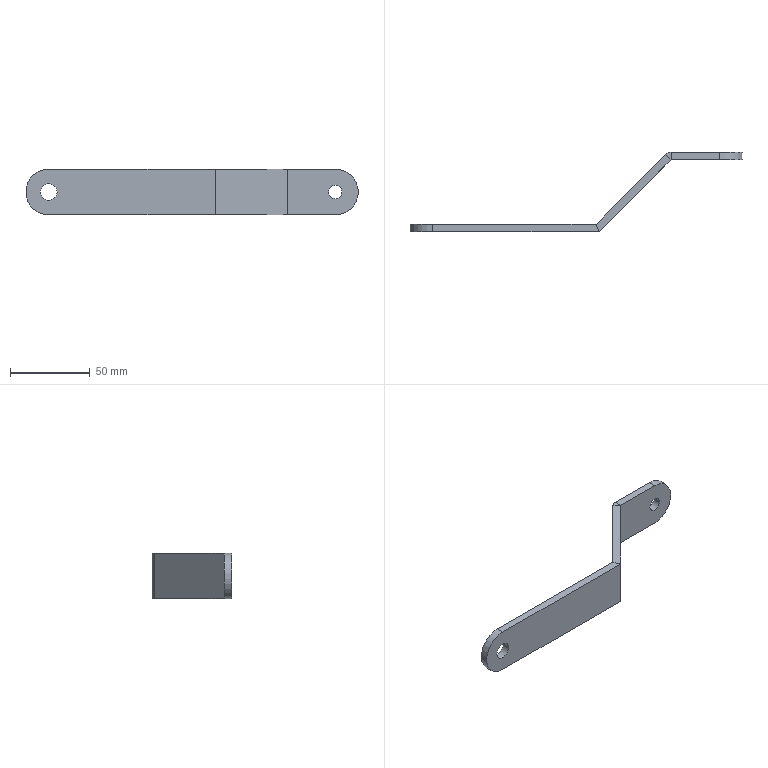Part | NX | features BREP 1 | 1 solid | 21 faces | box 207.715 x 49.664 x 28.575 mm | volume 29293 mm3 | plane 14 | cylinder 7 | commonest cylinder face diameters 8.204 x2 10.414 x2 28.575 x2 9.525 x1
STEP:
#1=CARTESIAN_POINT('',(118.364,0.,14.287));
#2=VERTEX_POINT('',#1);
#3=CARTESIAN_POINT('',(118.364,0.,-14.287));
#4=VERTEX_POINT('',#3);
#5=CARTESIAN_POINT('',(118.364,0.,14.287));
#6=DIRECTION('',(0.,0.,-1.));
#7=VECTOR('',#6,1000.);
#8=LINE('',#5,#7);
#9=EDGE_CURVE('',#2,#4,#8,.T.);
#10=ORIENTED_EDGE('',*,*,#9,.T.);
#11=CARTESIAN_POINT('',(163.265,44.901,-14.287));
#12=VERTEX_POINT('',#11);
#13=CARTESIAN_POINT('',(118.364,0.,-14.287));
#14=DIRECTION('',(0.7071,0.7071,0.));
#15=VECTOR('',#14,1000.);
#16=LINE('',#13,#15);
#17=EDGE_CURVE('',#4,#12,#16,.T.);
#18=ORIENTED_EDGE('',*,*,#17,.T.);
#19=CARTESIAN_POINT('',(163.265,44.901,14.287));
#20=VERTEX_POINT('',#19);
#21=CARTESIAN_POINT('',(163.265,44.901,14.287));
#22=DIRECTION('',(0.,0.,-1.));
#23=VECTOR('',#22,1000.);
#24=LINE('',#21,#23);
#25=EDGE_CURVE('',#20,#12,#24,.T.);
#26=ORIENTED_EDGE('',*,*,#25,.F.);
#27=CARTESIAN_POINT('',(118.364,0.,14.287));
#28=DIRECTION('',(0.7071,0.7071,0.));
#29=VECTOR('',#28,1000.);
#30=LINE('',#27,#29);
#31=EDGE_CURVE('',#2,#20,#30,.T.);
#32=ORIENTED_EDGE('',*,*,#31,.F.);
#33=EDGE_LOOP('',(#10,#18,#26,#32));
#34=FACE_BOUND('',#33,.T.);
#35=CARTESIAN_POINT('',(118.364,0.,14.287));
#36=DIRECTION('',(0.7071,-0.7071,0.));
#37=DIRECTION('',(0.,0.,-1.));
#38=AXIS2_PLACEMENT_3D('',#35,#36,#37);
#39=PLANE('',#38);
#40=ADVANCED_FACE('',(#34),#39,.T.);
#41=CARTESIAN_POINT('',(159.898,48.269,14.287));
#42=VERTEX_POINT('',#41);
#43=CARTESIAN_POINT('',(163.265,44.901,14.287));
#44=DIRECTION('',(-0.7071,0.7071,0.));
#45=VECTOR('',#44,1000.);
#46=LINE('',#43,#45);
#47=EDGE_CURVE('',#20,#42,#46,.T.);
#48=ORIENTED_EDGE('',*,*,#47,.T.);
#49=CARTESIAN_POINT('',(116.391,4.763,14.287));
#50=VERTEX_POINT('',#49);
#51=CARTESIAN_POINT('',(116.391,4.763,14.287));
#52=DIRECTION('',(0.7071,0.7071,0.));
#53=VECTOR('',#52,1000.);
#54=LINE('',#51,#53);
#55=EDGE_CURVE('',#50,#42,#54,.T.);
#56=ORIENTED_EDGE('',*,*,#55,.F.);
#57=CARTESIAN_POINT('',(118.364,0.,14.287));
#58=DIRECTION('',(-0.3827,0.9239,0.));
#59=VECTOR('',#58,1000.);
#60=LINE('',#57,#59);
#61=EDGE_CURVE('',#2,#50,#60,.T.);
#62=ORIENTED_EDGE('',*,*,#61,.F.);
#63=ORIENTED_EDGE('',*,*,#31,.T.);
#64=EDGE_LOOP('',(#48,#56,#62,#63));
#65=FACE_BOUND('',#64,.T.);
#66=CARTESIAN_POINT('',(139.48,24.483,14.287));
#67=DIRECTION('',(0.,0.,-1.));
#68=DIRECTION('',(0.,-1.,0.));
#69=AXIS2_PLACEMENT_3D('',#66,#67,#68);
#70=PLANE('',#69);
#71=ADVANCED_FACE('',(#65),#70,.F.);
#72=CARTESIAN_POINT('',(14.287,0.,14.287));
#73=VERTEX_POINT('',#72);
#74=CARTESIAN_POINT('',(14.287,0.,14.287));
#75=DIRECTION('',(1.,0.,0.));
#76=VECTOR('',#75,1000.);
#77=LINE('',#74,#76);
#78=EDGE_CURVE('',#73,#2,#77,.T.);
#79=ORIENTED_EDGE('',*,*,#78,.T.);
#80=ORIENTED_EDGE('',*,*,#61,.T.);
#81=CARTESIAN_POINT('',(14.287,4.763,14.287));
#82=VERTEX_POINT('',#81);
#83=CARTESIAN_POINT('',(14.287,4.763,14.287));
#84=DIRECTION('',(1.,0.,0.));
#85=VECTOR('',#84,1000.);
#86=LINE('',#83,#85);
#87=EDGE_CURVE('',#82,#50,#86,.T.);
#88=ORIENTED_EDGE('',*,*,#87,.F.);
#89=CARTESIAN_POINT('',(14.287,0.,14.287));
#90=DIRECTION('',(0.,1.,0.));
#91=VECTOR('',#90,1000.);
#92=LINE('',#89,#91);
#93=EDGE_CURVE('',#73,#82,#92,.T.);
#94=ORIENTED_EDGE('',*,*,#93,.F.);
#95=EDGE_LOOP('',(#79,#80,#88,#94));
#96=FACE_BOUND('',#95,.T.);
#97=CARTESIAN_POINT('',(58.689,2.381,14.287));
#98=DIRECTION('',(0.,0.,-1.));
#99=DIRECTION('',(0.,-1.,0.));
#100=AXIS2_PLACEMENT_3D('',#97,#98,#99);
#101=PLANE('',#100);
#102=ADVANCED_FACE('',(#96),#101,.F.);
#103=CARTESIAN_POINT('',(14.287,4.763,-14.287));
#104=VERTEX_POINT('',#103);
#105=CARTESIAN_POINT('',(14.287,4.763,0.));
#106=DIRECTION('',(0.,1.,0.));
#107=DIRECTION('',(0.,0.,-1.));
#108=AXIS2_PLACEMENT_3D('',#105,#106,#107);
#109=CIRCLE('',#108,14.287);
#110=EDGE_CURVE('',#104,#82,#109,.T.);
#111=ORIENTED_EDGE('',*,*,#110,.F.);
#112=CARTESIAN_POINT('',(14.287,0.,-14.287));
#113=VERTEX_POINT('',#112);
#114=CARTESIAN_POINT('',(14.287,0.,-14.287));
#115=DIRECTION('',(0.,1.,0.));
#116=VECTOR('',#115,1000.);
#117=LINE('',#114,#116);
#118=EDGE_CURVE('',#113,#104,#117,.T.);
#119=ORIENTED_EDGE('',*,*,#118,.F.);
#120=CARTESIAN_POINT('',(14.287,0.,0.));
#121=DIRECTION('',(0.,-1.,0.));
#122=DIRECTION('',(0.,0.,1.));
#123=AXIS2_PLACEMENT_3D('',#120,#121,#122);
#124=CIRCLE('',#123,14.287);
#125=EDGE_CURVE('',#73,#113,#124,.T.);
#126=ORIENTED_EDGE('',*,*,#125,.F.);
#127=ORIENTED_EDGE('',*,*,#93,.T.);
#128=EDGE_LOOP('',(#111,#119,#126,#127));
#129=FACE_BOUND('',#128,.T.);
#130=CARTESIAN_POINT('',(14.287,-0.3376,0.));
#131=DIRECTION('',(0.,1.,0.));
#132=DIRECTION('',(0.,0.,1.));
#133=AXIS2_PLACEMENT_3D('',#130,#131,#132);
#134=CYLINDRICAL_SURFACE('',#133,14.287);
#135=ADVANCED_FACE('',(#129),#134,.T.);
#136=CARTESIAN_POINT('',(14.287,0.,-14.287));
#137=DIRECTION('',(1.,0.,0.));
#138=VECTOR('',#137,1000.);
#139=LINE('',#136,#138);
#140=EDGE_CURVE('',#113,#4,#139,.T.);
#141=ORIENTED_EDGE('',*,*,#140,.T.);
#142=ORIENTED_EDGE('',*,*,#9,.F.);
#143=ORIENTED_EDGE('',*,*,#78,.F.);
#144=ORIENTED_EDGE('',*,*,#125,.T.);
#145=EDGE_LOOP('',(#141,#142,#143,#144));
#146=FACE_BOUND('',#145,.T.);
#147=CARTESIAN_POINT('',(19.494,0.,0.));
#148=VERTEX_POINT('',#147);
#149=CARTESIAN_POINT('',(9.081,0.,0.));
#150=VERTEX_POINT('',#149);
#151=CARTESIAN_POINT('',(14.287,0.,0.));
#152=DIRECTION('',(0.,1.,0.));
#153=DIRECTION('',(1.,0.,0.));
#154=AXIS2_PLACEMENT_3D('',#151,#152,#153);
#155=CIRCLE('',#154,5.207);
#156=EDGE_CURVE('',#148,#150,#155,.T.);
#157=ORIENTED_EDGE('',*,*,#156,.T.);
#158=CARTESIAN_POINT('',(14.287,0.,0.));
#159=DIRECTION('',(0.,1.,0.));
#160=DIRECTION('',(-1.,0.,0.));
#161=AXIS2_PLACEMENT_3D('',#158,#159,#160);
#162=CIRCLE('',#161,5.207);
#163=EDGE_CURVE('',#150,#148,#162,.T.);
#164=ORIENTED_EDGE('',*,*,#163,.T.);
#165=EDGE_LOOP('',(#157,#164));
#166=FACE_BOUND('',#165,.T.);
#167=CARTESIAN_POINT('',(0.,0.,14.287));
#168=DIRECTION('',(0.,-1.,0.));
#169=DIRECTION('',(0.,0.,-1.));
#170=AXIS2_PLACEMENT_3D('',#167,#168,#169);
#171=PLANE('',#170);
#172=ADVANCED_FACE('',(#146,#166),#171,.T.);
#173=CARTESIAN_POINT('',(116.391,4.763,-14.287));
#174=VERTEX_POINT('',#173);
#175=CARTESIAN_POINT('',(14.287,4.763,-14.287));
#176=DIRECTION('',(1.,0.,0.));
#177=VECTOR('',#176,1000.);
#178=LINE('',#175,#177);
#179=EDGE_CURVE('',#104,#174,#178,.T.);
#180=ORIENTED_EDGE('',*,*,#179,.T.);
#181=CARTESIAN_POINT('',(118.364,0.,-14.287));
#182=DIRECTION('',(-0.3827,0.9239,0.));
#183=VECTOR('',#182,1000.);
#184=LINE('',#181,#183);
#185=EDGE_CURVE('',#4,#174,#184,.T.);
#186=ORIENTED_EDGE('',*,*,#185,.F.);
#187=ORIENTED_EDGE('',*,*,#140,.F.);
#188=ORIENTED_EDGE('',*,*,#118,.T.);
#189=EDGE_LOOP('',(#180,#186,#187,#188));
#190=FACE_BOUND('',#189,.T.);
#191=CARTESIAN_POINT('',(58.689,2.381,-14.287));
#192=DIRECTION('',(0.,0.,-1.));
#193=DIRECTION('',(0.,-1.,0.));
#194=AXIS2_PLACEMENT_3D('',#191,#192,#193);
#195=PLANE('',#194);
#196=ADVANCED_FACE('',(#190),#195,.T.);
#197=ORIENTED_EDGE('',*,*,#185,.T.);
#198=CARTESIAN_POINT('',(159.898,48.269,-14.287));
#199=VERTEX_POINT('',#198);
#200=CARTESIAN_POINT('',(116.391,4.763,-14.287));
#201=DIRECTION('',(0.7071,0.7071,0.));
#202=VECTOR('',#201,1000.);
#203=LINE('',#200,#202);
#204=EDGE_CURVE('',#174,#199,#203,.T.);
#205=ORIENTED_EDGE('',*,*,#204,.T.);
#206=CARTESIAN_POINT('',(163.265,44.901,-14.287));
#207=DIRECTION('',(-0.7071,0.7071,0.));
#208=VECTOR('',#207,1000.);
#209=LINE('',#206,#208);
#210=EDGE_CURVE('',#12,#199,#209,.T.);
#211=ORIENTED_EDGE('',*,*,#210,.F.);
#212=ORIENTED_EDGE('',*,*,#17,.F.);
#213=EDGE_LOOP('',(#197,#205,#211,#212));
#214=FACE_BOUND('',#213,.T.);
#215=CARTESIAN_POINT('',(139.48,24.483,-14.287));
#216=DIRECTION('',(0.,0.,-1.));
#217=DIRECTION('',(0.,-1.,0.));
#218=AXIS2_PLACEMENT_3D('',#215,#216,#217);
#219=PLANE('',#218);
#220=ADVANCED_FACE('',(#214),#219,.T.);
#221=CARTESIAN_POINT('',(163.265,49.664,-14.287));
#222=VERTEX_POINT('',#221);
#223=CARTESIAN_POINT('',(163.265,44.901,-14.287));
#224=DIRECTION('',(0.,0.,-1.));
#225=DIRECTION('',(-0.7071,0.7071,0.));
#226=AXIS2_PLACEMENT_3D('',#223,#224,#225);
#227=CIRCLE('',#226,4.763);
#228=EDGE_CURVE('',#199,#222,#227,.T.);
#229=ORIENTED_EDGE('',*,*,#228,.T.);
#230=CARTESIAN_POINT('',(163.265,44.901,-14.287));
#231=DIRECTION('',(0.,1.,0.));
#232=VECTOR('',#231,1000.);
#233=LINE('',#230,#232);
#234=EDGE_CURVE('',#12,#222,#233,.T.);
#235=ORIENTED_EDGE('',*,*,#234,.F.);
#236=ORIENTED_EDGE('',*,*,#210,.T.);
#237=EDGE_LOOP('',(#229,#235,#236));
#238=FACE_BOUND('',#237,.T.);
#239=CARTESIAN_POINT('',(162.354,47.101,-14.287));
#240=DIRECTION('',(0.,0.,-1.));
#241=DIRECTION('',(0.,-1.,0.));
#242=AXIS2_PLACEMENT_3D('',#239,#240,#241);
#243=PLANE('',#242);
#244=ADVANCED_FACE('',(#238),#243,.T.);
#245=CARTESIAN_POINT('',(193.428,44.901,-14.287));
#246=VERTEX_POINT('',#245);
#247=CARTESIAN_POINT('',(163.265,44.901,-14.287));
#248=DIRECTION('',(1.,0.,0.));
#249=VECTOR('',#248,1000.);
#250=LINE('',#247,#249);
#251=EDGE_CURVE('',#12,#246,#250,.T.);
#252=ORIENTED_EDGE('',*,*,#251,.F.);
#253=ORIENTED_EDGE('',*,*,#234,.T.);
#254=CARTESIAN_POINT('',(193.428,49.664,-14.287));
#255=VERTEX_POINT('',#254);
#256=CARTESIAN_POINT('',(163.265,49.664,-14.287));
#257=DIRECTION('',(1.,0.,0.));
#258=VECTOR('',#257,1000.);
#259=LINE('',#256,#258);
#260=EDGE_CURVE('',#222,#255,#259,.T.);
#261=ORIENTED_EDGE('',*,*,#260,.T.);
#262=CARTESIAN_POINT('',(193.428,49.664,-14.287));
#263=DIRECTION('',(0.,-1.,0.));
#264=VECTOR('',#263,1000.);
#265=LINE('',#262,#264);
#266=EDGE_CURVE('',#255,#246,#265,.T.);
#267=ORIENTED_EDGE('',*,*,#266,.T.);
#268=EDGE_LOOP('',(#252,#253,#261,#267));
#269=FACE_BOUND('',#268,.T.);
#270=CARTESIAN_POINT('',(185.49,47.283,-14.287));
#271=DIRECTION('',(0.,0.,-1.));
#272=DIRECTION('',(0.,-1.,0.));
#273=AXIS2_PLACEMENT_3D('',#270,#271,#272);
#274=PLANE('',#273);
#275=ADVANCED_FACE('',(#269),#274,.T.);
#276=CARTESIAN_POINT('',(193.428,44.901,14.287));
#277=VERTEX_POINT('',#276);
#278=CARTESIAN_POINT('',(193.428,44.901,0.));
#279=DIRECTION('',(0.,-1.,0.));
#280=DIRECTION('',(0.,0.,-1.));
#281=AXIS2_PLACEMENT_3D('',#278,#279,#280);
#282=CIRCLE('',#281,14.287);
#283=EDGE_CURVE('',#246,#277,#282,.T.);
#284=ORIENTED_EDGE('',*,*,#283,.F.);
#285=ORIENTED_EDGE('',*,*,#266,.F.);
#286=CARTESIAN_POINT('',(193.428,49.664,14.287));
#287=VERTEX_POINT('',#286);
#288=CARTESIAN_POINT('',(193.428,49.664,0.));
#289=DIRECTION('',(0.,1.,0.));
#290=DIRECTION('',(0.,0.,1.));
#291=AXIS2_PLACEMENT_3D('',#288,#289,#290);
#292=CIRCLE('',#291,14.287);
#293=EDGE_CURVE('',#287,#255,#292,.T.);
#294=ORIENTED_EDGE('',*,*,#293,.F.);
#295=CARTESIAN_POINT('',(193.428,49.664,14.287));
#296=DIRECTION('',(0.,-1.,0.));
#297=VECTOR('',#296,1000.);
#298=LINE('',#295,#297);
#299=EDGE_CURVE('',#287,#277,#298,.T.);
#300=ORIENTED_EDGE('',*,*,#299,.T.);
#301=EDGE_LOOP('',(#284,#285,#294,#300));
#302=FACE_BOUND('',#301,.T.);
#303=CARTESIAN_POINT('',(193.428,49.952,0.));
#304=DIRECTION('',(0.,-1.,0.));
#305=DIRECTION('',(0.,0.,1.));
#306=AXIS2_PLACEMENT_3D('',#303,#304,#305);
#307=CYLINDRICAL_SURFACE('',#306,14.287);
#308=ADVANCED_FACE('',(#302),#307,.T.);
#309=CARTESIAN_POINT('',(163.265,49.664,14.287));
#310=VERTEX_POINT('',#309);
#311=CARTESIAN_POINT('',(163.265,49.664,14.287));
#312=DIRECTION('',(1.,0.,0.));
#313=VECTOR('',#312,1000.);
#314=LINE('',#311,#313);
#315=EDGE_CURVE('',#310,#287,#314,.T.);
#316=ORIENTED_EDGE('',*,*,#315,.F.);
#317=CARTESIAN_POINT('',(163.265,44.901,14.287));
#318=DIRECTION('',(0.,1.,0.));
#319=VECTOR('',#318,1000.);
#320=LINE('',#317,#319);
#321=EDGE_CURVE('',#20,#310,#320,.T.);
#322=ORIENTED_EDGE('',*,*,#321,.F.);
#323=CARTESIAN_POINT('',(163.265,44.901,14.287));
#324=DIRECTION('',(1.,0.,0.));
#325=VECTOR('',#324,1000.);
#326=LINE('',#323,#325);
#327=EDGE_CURVE('',#20,#277,#326,.T.);
#328=ORIENTED_EDGE('',*,*,#327,.T.);
#329=ORIENTED_EDGE('',*,*,#299,.F.);
#330=EDGE_LOOP('',(#316,#322,#328,#329));
#331=FACE_BOUND('',#330,.T.);
#332=CARTESIAN_POINT('',(185.49,47.283,14.287));
#333=DIRECTION('',(0.,0.,-1.));
#334=DIRECTION('',(0.,-1.,0.));
#335=AXIS2_PLACEMENT_3D('',#332,#333,#334);
#336=PLANE('',#335);
#337=ADVANCED_FACE('',(#331),#336,.F.);
#338=ORIENTED_EDGE('',*,*,#327,.F.);
#339=ORIENTED_EDGE('',*,*,#25,.T.);
#340=ORIENTED_EDGE('',*,*,#251,.T.);
#341=ORIENTED_EDGE('',*,*,#283,.T.);
#342=EDGE_LOOP('',(#338,#339,#340,#341));
#343=FACE_BOUND('',#342,.T.);
#344=CARTESIAN_POINT('',(197.53,44.901,0.));
#345=VERTEX_POINT('',#344);
#346=CARTESIAN_POINT('',(189.326,44.901,0.));
#347=VERTEX_POINT('',#346);
#348=CARTESIAN_POINT('',(193.428,44.901,0.));
#349=DIRECTION('',(0.,1.,0.));
#350=DIRECTION('',(1.,0.,0.));
#351=AXIS2_PLACEMENT_3D('',#348,#349,#350);
#352=CIRCLE('',#351,4.102);
#353=EDGE_CURVE('',#345,#347,#352,.T.);
#354=ORIENTED_EDGE('',*,*,#353,.T.);
#355=CARTESIAN_POINT('',(193.428,44.901,0.));
#356=DIRECTION('',(0.,1.,0.));
#357=DIRECTION('',(-1.,0.,0.));
#358=AXIS2_PLACEMENT_3D('',#355,#356,#357);
#359=CIRCLE('',#358,4.102);
#360=EDGE_CURVE('',#347,#345,#359,.T.);
#361=ORIENTED_EDGE('',*,*,#360,.T.);
#362=EDGE_LOOP('',(#354,#361));
#363=FACE_BOUND('',#362,.T.);
#364=CARTESIAN_POINT('',(163.265,44.901,14.287));
#365=DIRECTION('',(0.,-1.,0.));
#366=DIRECTION('',(0.,0.,-1.));
#367=AXIS2_PLACEMENT_3D('',#364,#365,#366);
#368=PLANE('',#367);
#369=ADVANCED_FACE('',(#343,#363),#368,.T.);
#370=CARTESIAN_POINT('',(197.53,49.664,0.));
#371=VERTEX_POINT('',#370);
#372=CARTESIAN_POINT('',(197.53,49.664,0.));
#373=DIRECTION('',(0.,-1.,0.));
#374=VECTOR('',#373,1000.);
#375=LINE('',#372,#374);
#376=EDGE_CURVE('',#345,#371,#375,.F.);
#377=ORIENTED_EDGE('',*,*,#376,.F.);
#378=ORIENTED_EDGE('',*,*,#360,.F.);
#379=CARTESIAN_POINT('',(189.326,49.664,0.));
#380=VERTEX_POINT('',#379);
#381=CARTESIAN_POINT('',(189.326,49.664,0.));
#382=DIRECTION('',(0.,-1.,0.));
#383=VECTOR('',#382,1000.);
#384=LINE('',#381,#383);
#385=EDGE_CURVE('',#347,#380,#384,.F.);
#386=ORIENTED_EDGE('',*,*,#385,.T.);
#387=CARTESIAN_POINT('',(193.428,49.664,0.));
#388=DIRECTION('',(0.,1.,0.));
#389=DIRECTION('',(-1.,0.,0.));
#390=AXIS2_PLACEMENT_3D('',#387,#388,#389);
#391=CIRCLE('',#390,4.102);
#392=EDGE_CURVE('',#380,#371,#391,.T.);
#393=ORIENTED_EDGE('',*,*,#392,.T.);
#394=EDGE_LOOP('',(#377,#378,#386,#393));
#395=FACE_BOUND('',#394,.T.);
#396=CARTESIAN_POINT('',(193.428,47.283,0.));
#397=DIRECTION('',(0.,1.,0.));
#398=DIRECTION('',(-1.,0.,0.));
#399=AXIS2_PLACEMENT_3D('',#396,#397,#398);
#400=CYLINDRICAL_SURFACE('',#399,4.102);
#401=ADVANCED_FACE('',(#395),#400,.F.);
#402=ORIENTED_EDGE('',*,*,#260,.F.);
#403=CARTESIAN_POINT('',(163.265,49.664,14.287));
#404=DIRECTION('',(0.,0.,-1.));
#405=VECTOR('',#404,1000.);
#406=LINE('',#403,#405);
#407=EDGE_CURVE('',#310,#222,#406,.T.);
#408=ORIENTED_EDGE('',*,*,#407,.F.);
#409=ORIENTED_EDGE('',*,*,#315,.T.);
#410=ORIENTED_EDGE('',*,*,#293,.T.);
#411=EDGE_LOOP('',(#402,#408,#409,#410));
#412=FACE_BOUND('',#411,.T.);
#413=CARTESIAN_POINT('',(193.428,49.664,0.));
#414=DIRECTION('',(0.,1.,0.));
#415=DIRECTION('',(1.,0.,0.));
#416=AXIS2_PLACEMENT_3D('',#413,#414,#415);
#417=CIRCLE('',#416,4.102);
#418=EDGE_CURVE('',#371,#380,#417,.T.);
#419=ORIENTED_EDGE('',*,*,#418,.F.);
#420=ORIENTED_EDGE('',*,*,#392,.F.);
#421=EDGE_LOOP('',(#419,#420));
#422=FACE_BOUND('',#421,.T.);
#423=CARTESIAN_POINT('',(163.265,49.664,14.287));
#424=DIRECTION('',(0.,-1.,0.));
#425=DIRECTION('',(0.,0.,-1.));
#426=AXIS2_PLACEMENT_3D('',#423,#424,#425);
#427=PLANE('',#426);
#428=ADVANCED_FACE('',(#412,#422),#427,.F.);
#429=ORIENTED_EDGE('',*,*,#228,.F.);
#430=CARTESIAN_POINT('',(159.898,48.269,14.287));
#431=DIRECTION('',(0.,0.,-1.));
#432=VECTOR('',#431,1000.);
#433=LINE('',#430,#432);
#434=EDGE_CURVE('',#42,#199,#433,.T.);
#435=ORIENTED_EDGE('',*,*,#434,.F.);
#436=CARTESIAN_POINT('',(163.265,44.901,14.287));
#437=DIRECTION('',(0.,0.,1.));
#438=DIRECTION('',(0.,1.,0.));
#439=AXIS2_PLACEMENT_3D('',#436,#437,#438);
#440=CIRCLE('',#439,4.763);
#441=EDGE_CURVE('',#310,#42,#440,.T.);
#442=ORIENTED_EDGE('',*,*,#441,.F.);
#443=ORIENTED_EDGE('',*,*,#407,.T.);
#444=EDGE_LOOP('',(#429,#435,#442,#443));
#445=FACE_BOUND('',#444,.T.);
#446=CARTESIAN_POINT('',(163.265,44.901,14.287));
#447=DIRECTION('',(0.,0.,-1.));
#448=DIRECTION('',(0.,1.,0.));
#449=AXIS2_PLACEMENT_3D('',#446,#447,#448);
#450=CYLINDRICAL_SURFACE('',#449,4.763);
#451=ADVANCED_FACE('',(#445),#450,.T.);
#452=ORIENTED_EDGE('',*,*,#441,.T.);
#453=ORIENTED_EDGE('',*,*,#47,.F.);
#454=ORIENTED_EDGE('',*,*,#321,.T.);
#455=EDGE_LOOP('',(#452,#453,#454));
#456=FACE_BOUND('',#455,.T.);
#457=CARTESIAN_POINT('',(162.354,47.101,14.287));
#458=DIRECTION('',(0.,0.,1.));
#459=DIRECTION('',(1.,0.,0.));
#460=AXIS2_PLACEMENT_3D('',#457,#458,#459);
#461=PLANE('',#460);
#462=ADVANCED_FACE('',(#456),#461,.T.);
#463=ORIENTED_EDGE('',*,*,#434,.T.);
#464=ORIENTED_EDGE('',*,*,#204,.F.);
#465=CARTESIAN_POINT('',(116.391,4.763,14.287));
#466=DIRECTION('',(0.,0.,-1.));
#467=VECTOR('',#466,1000.);
#468=LINE('',#465,#467);
#469=EDGE_CURVE('',#50,#174,#468,.T.);
#470=ORIENTED_EDGE('',*,*,#469,.F.);
#471=ORIENTED_EDGE('',*,*,#55,.T.);
#472=EDGE_LOOP('',(#463,#464,#470,#471));
#473=FACE_BOUND('',#472,.T.);
#474=CARTESIAN_POINT('',(114.996,3.368,14.287));
#475=DIRECTION('',(0.7071,-0.7071,0.));
#476=DIRECTION('',(0.,0.,-1.));
#477=AXIS2_PLACEMENT_3D('',#474,#475,#476);
#478=PLANE('',#477);
#479=ADVANCED_FACE('',(#473),#478,.F.);
#480=ORIENTED_EDGE('',*,*,#87,.T.);
#481=ORIENTED_EDGE('',*,*,#469,.T.);
#482=ORIENTED_EDGE('',*,*,#179,.F.);
#483=ORIENTED_EDGE('',*,*,#110,.T.);
#484=EDGE_LOOP('',(#480,#481,#482,#483));
#485=FACE_BOUND('',#484,.T.);
#486=CARTESIAN_POINT('',(19.494,4.763,0.));
#487=VERTEX_POINT('',#486);
#488=CARTESIAN_POINT('',(9.081,4.763,0.));
#489=VERTEX_POINT('',#488);
#490=CARTESIAN_POINT('',(14.287,4.763,0.));
#491=DIRECTION('',(0.,1.,0.));
#492=DIRECTION('',(1.,0.,0.));
#493=AXIS2_PLACEMENT_3D('',#490,#491,#492);
#494=CIRCLE('',#493,5.207);
#495=EDGE_CURVE('',#487,#489,#494,.T.);
#496=ORIENTED_EDGE('',*,*,#495,.F.);
#497=CARTESIAN_POINT('',(14.287,4.763,0.));
#498=DIRECTION('',(0.,1.,0.));
#499=DIRECTION('',(-1.,0.,0.));
#500=AXIS2_PLACEMENT_3D('',#497,#498,#499);
#501=CIRCLE('',#500,5.207);
#502=EDGE_CURVE('',#489,#487,#501,.T.);
#503=ORIENTED_EDGE('',*,*,#502,.F.);
#504=EDGE_LOOP('',(#496,#503));
#505=FACE_BOUND('',#504,.T.);
#506=CARTESIAN_POINT('',(0.,4.763,14.287));
#507=DIRECTION('',(0.,-1.,0.));
#508=DIRECTION('',(0.,0.,-1.));
#509=AXIS2_PLACEMENT_3D('',#506,#507,#508);
#510=PLANE('',#509);
#511=ADVANCED_FACE('',(#485,#505),#510,.F.);
#512=CARTESIAN_POINT('',(19.494,4.763,0.));
#513=DIRECTION('',(0.,-1.,0.));
#514=VECTOR('',#513,1000.);
#515=LINE('',#512,#514);
#516=EDGE_CURVE('',#148,#487,#515,.F.);
#517=ORIENTED_EDGE('',*,*,#516,.F.);
#518=ORIENTED_EDGE('',*,*,#163,.F.);
#519=CARTESIAN_POINT('',(9.081,4.763,0.));
#520=DIRECTION('',(0.,-1.,0.));
#521=VECTOR('',#520,1000.);
#522=LINE('',#519,#521);
#523=EDGE_CURVE('',#150,#489,#522,.F.);
#524=ORIENTED_EDGE('',*,*,#523,.T.);
#525=ORIENTED_EDGE('',*,*,#502,.T.);
#526=EDGE_LOOP('',(#517,#518,#524,#525));
#527=FACE_BOUND('',#526,.T.);
#528=CARTESIAN_POINT('',(14.287,2.381,0.));
#529=DIRECTION('',(0.,1.,0.));
#530=DIRECTION('',(-1.,0.,0.));
#531=AXIS2_PLACEMENT_3D('',#528,#529,#530);
#532=CYLINDRICAL_SURFACE('',#531,5.207);
#533=ADVANCED_FACE('',(#527),#532,.F.);
#534=ORIENTED_EDGE('',*,*,#523,.F.);
#535=ORIENTED_EDGE('',*,*,#156,.F.);
#536=ORIENTED_EDGE('',*,*,#516,.T.);
#537=ORIENTED_EDGE('',*,*,#495,.T.);
#538=EDGE_LOOP('',(#534,#535,#536,#537));
#539=FACE_BOUND('',#538,.T.);
#540=CARTESIAN_POINT('',(14.287,2.381,0.));
#541=DIRECTION('',(0.,1.,0.));
#542=DIRECTION('',(1.,0.,0.));
#543=AXIS2_PLACEMENT_3D('',#540,#541,#542);
#544=CYLINDRICAL_SURFACE('',#543,5.207);
#545=ADVANCED_FACE('',(#539),#544,.F.);
#546=ORIENTED_EDGE('',*,*,#385,.F.);
#547=ORIENTED_EDGE('',*,*,#353,.F.);
#548=ORIENTED_EDGE('',*,*,#376,.T.);
#549=ORIENTED_EDGE('',*,*,#418,.T.);
#550=EDGE_LOOP('',(#546,#547,#548,#549));
#551=FACE_BOUND('',#550,.T.);
#552=CARTESIAN_POINT('',(193.428,47.283,0.));
#553=DIRECTION('',(0.,1.,0.));
#554=DIRECTION('',(1.,0.,0.));
#555=AXIS2_PLACEMENT_3D('',#552,#553,#554);
#556=CYLINDRICAL_SURFACE('',#555,4.102);
#557=ADVANCED_FACE('',(#551),#556,.F.);
#558=CLOSED_SHELL('',(#40,#71,#102,#135,#172,#196,#220,#244,#275,#308,#337,#369,#401,#428,#451,#462,#479,#511,#533,#545,#557));
#559=MANIFOLD_SOLID_BREP('',#558);
#560=(LENGTH_UNIT()NAMED_UNIT(*)SI_UNIT(.MILLI.,.METRE.));
#561=UNCERTAINTY_MEASURE_WITH_UNIT(LENGTH_MEASURE(0.00001),#560,'','');
#562=(NAMED_UNIT(*)PLANE_ANGLE_UNIT()SI_UNIT($,.RADIAN.));
#563=(NAMED_UNIT(*)SI_UNIT($,.STERADIAN.)SOLID_ANGLE_UNIT());
#564=(GEOMETRIC_REPRESENTATION_CONTEXT(3)GLOBAL_UNCERTAINTY_ASSIGNED_CONTEXT((#561))GLOBAL_UNIT_ASSIGNED_CONTEXT((#560,#562,#563))REPRESENTATION_CONTEXT('',''));
#565=ADVANCED_BREP_SHAPE_REPRESENTATION('',(#559),#564);